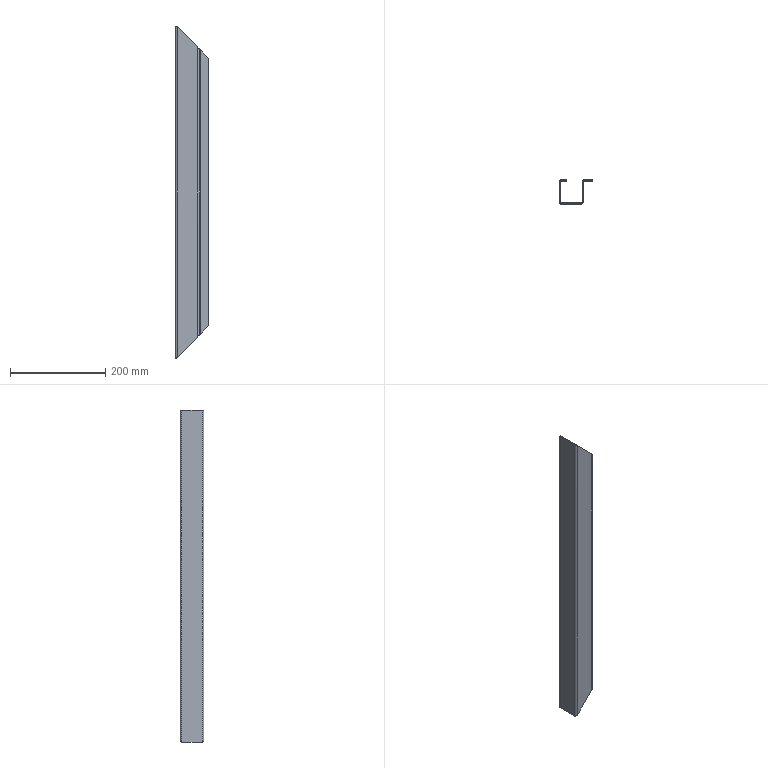Part | STEP file | 750038466 | 1 solid | 38 faces | box 70 x 50 x 696 mm | volume 223669 mm3 | plane 22 | cylinder 8 | spline 8 | commonest cylinder face diameters 4 x4 8 x4
STEP:
#1=CARTESIAN_POINT('',(0.,46.,-348.));
#2=VERTEX_POINT('',#1);
#3=CARTESIAN_POINT('',(0.,4.,-348.));
#4=VERTEX_POINT('',#3);
#5=CARTESIAN_POINT('',(0.,0.,-348.));
#6=DIRECTION('',(0.,-1.,0.));
#7=VECTOR('',#6,1000.);
#8=LINE('',#5,#7);
#9=EDGE_CURVE('',#2,#4,#8,.T.);
#10=ORIENTED_EDGE('',*,*,#9,.T.);
#11=CARTESIAN_POINT('',(0.,4.,348.));
#12=VERTEX_POINT('',#11);
#13=CARTESIAN_POINT('',(0.,4.,350.));
#14=DIRECTION('',(0.,0.,1.));
#15=VECTOR('',#14,1000.);
#16=LINE('',#13,#15);
#17=EDGE_CURVE('',#4,#12,#16,.T.);
#18=ORIENTED_EDGE('',*,*,#17,.T.);
#19=CARTESIAN_POINT('',(0.,46.,348.));
#20=VERTEX_POINT('',#19);
#21=CARTESIAN_POINT('',(0.,0.,348.));
#22=DIRECTION('',(0.,1.,0.));
#23=VECTOR('',#22,1000.);
#24=LINE('',#21,#23);
#25=EDGE_CURVE('',#12,#20,#24,.T.);
#26=ORIENTED_EDGE('',*,*,#25,.T.);
#27=CARTESIAN_POINT('',(0.,46.,350.));
#28=DIRECTION('',(0.,0.,-1.));
#29=VECTOR('',#28,1000.);
#30=LINE('',#27,#29);
#31=EDGE_CURVE('',#20,#2,#30,.T.);
#32=ORIENTED_EDGE('',*,*,#31,.T.);
#33=EDGE_LOOP('',(#10,#18,#26,#32));
#34=FACE_OUTER_BOUND('',#33,.T.);
#35=CARTESIAN_POINT('',(0.,0.,350.));
#36=DIRECTION('',(-1.,0.,0.));
#37=DIRECTION('',(0.,-1.,0.));
#38=AXIS2_PLACEMENT_3D('',#35,#36,#37);
#39=PLANE('',#38);
#40=ADVANCED_FACE('',(#34),#39,.T.);
#41=CARTESIAN_POINT('',(4.,0.,-346.));
#42=VERTEX_POINT('',#41);
#43=CARTESIAN_POINT('',(0.,4.,-348.));
#44=CARTESIAN_POINT('',(0.,2.,-348.));
#45=CARTESIAN_POINT('',(1.333,0.,-347.333));
#46=CARTESIAN_POINT('',(4.,0.,-346.));
#47=(BOUNDED_CURVE()B_SPLINE_CURVE(3,(#43,#44,#45,#46),.UNSPECIFIED.,.F.,.F.)B_SPLINE_CURVE_WITH_KNOTS((4,4),(0.,0.006692),.UNSPECIFIED.)CURVE()GEOMETRIC_REPRESENTATION_ITEM()RATIONAL_B_SPLINE_CURVE((1.,0.6667,0.5,0.5))REPRESENTATION_ITEM(''));
#48=EDGE_CURVE('',#4,#42,#47,.T.);
#49=ORIENTED_EDGE('',*,*,#48,.T.);
#50=CARTESIAN_POINT('',(4.,0.,346.));
#51=VERTEX_POINT('',#50);
#52=CARTESIAN_POINT('',(4.,0.,350.));
#53=DIRECTION('',(0.,0.,1.));
#54=VECTOR('',#53,1000.);
#55=LINE('',#52,#54);
#56=EDGE_CURVE('',#42,#51,#55,.T.);
#57=ORIENTED_EDGE('',*,*,#56,.T.);
#58=CARTESIAN_POINT('',(4.,0.,346.));
#59=CARTESIAN_POINT('',(1.333,0.,347.333));
#60=CARTESIAN_POINT('',(0.,2.,348.));
#61=CARTESIAN_POINT('',(0.,4.,348.));
#62=(BOUNDED_CURVE()B_SPLINE_CURVE(3,(#58,#59,#60,#61),.UNSPECIFIED.,.F.,.F.)B_SPLINE_CURVE_WITH_KNOTS((4,4),(0.,0.006641),.UNSPECIFIED.)CURVE()GEOMETRIC_REPRESENTATION_ITEM()RATIONAL_B_SPLINE_CURVE((0.5,0.5,0.6667,1.))REPRESENTATION_ITEM(''));
#63=EDGE_CURVE('',#51,#12,#62,.T.);
#64=ORIENTED_EDGE('',*,*,#63,.T.);
#65=ORIENTED_EDGE('',*,*,#17,.F.);
#66=EDGE_LOOP('',(#49,#57,#64,#65));
#67=FACE_OUTER_BOUND('',#66,.T.);
#68=CARTESIAN_POINT('',(4.,4.,350.));
#69=DIRECTION('',(0.,0.,-1.));
#70=DIRECTION('',(-1.,0.,0.));
#71=AXIS2_PLACEMENT_3D('',#68,#69,#70);
#72=CYLINDRICAL_SURFACE('',#71,4.);
#73=ADVANCED_FACE('',(#67),#72,.T.);
#74=CARTESIAN_POINT('',(2.,46.,-348.));
#75=VERTEX_POINT('',#74);
#76=CARTESIAN_POINT('',(2.,46.,-348.));
#77=DIRECTION('',(-1.,0.,0.));
#78=VECTOR('',#77,1000.);
#79=LINE('',#76,#78);
#80=EDGE_CURVE('',#75,#2,#79,.T.);
#81=ORIENTED_EDGE('',*,*,#80,.F.);
#82=CARTESIAN_POINT('',(2.,4.,-348.));
#83=VERTEX_POINT('',#82);
#84=CARTESIAN_POINT('',(2.,0.,-348.));
#85=DIRECTION('',(0.,1.,0.));
#86=VECTOR('',#85,1000.);
#87=LINE('',#84,#86);
#88=EDGE_CURVE('',#83,#75,#87,.T.);
#89=ORIENTED_EDGE('',*,*,#88,.F.);
#90=CARTESIAN_POINT('',(2.,4.,-348.));
#91=DIRECTION('',(1.,0.,0.));
#92=VECTOR('',#91,1000.);
#93=LINE('',#90,#92);
#94=EDGE_CURVE('',#4,#83,#93,.T.);
#95=ORIENTED_EDGE('',*,*,#94,.F.);
#96=ORIENTED_EDGE('',*,*,#9,.F.);
#97=EDGE_LOOP('',(#81,#89,#95,#96));
#98=FACE_OUTER_BOUND('',#97,.T.);
#99=CARTESIAN_POINT('',(2.,0.,-348.));
#100=DIRECTION('',(0.,0.,1.));
#101=DIRECTION('',(0.,-1.,0.));
#102=AXIS2_PLACEMENT_3D('',#99,#100,#101);
#103=PLANE('',#102);
#104=ADVANCED_FACE('',(#98),#103,.F.);
#105=CARTESIAN_POINT('',(4.,50.,-346.));
#106=VERTEX_POINT('',#105);
#107=CARTESIAN_POINT('',(4.,50.,-346.));
#108=CARTESIAN_POINT('',(1.333,50.,-347.333));
#109=CARTESIAN_POINT('',(0.,48.,-348.));
#110=CARTESIAN_POINT('',(0.,46.,-348.));
#111=(BOUNDED_CURVE()B_SPLINE_CURVE(3,(#107,#108,#109,#110),.UNSPECIFIED.,.F.,.F.)B_SPLINE_CURVE_WITH_KNOTS((4,4),(0.,0.006641),.UNSPECIFIED.)CURVE()GEOMETRIC_REPRESENTATION_ITEM()RATIONAL_B_SPLINE_CURVE((0.5,0.5,0.6667,1.))REPRESENTATION_ITEM(''));
#112=EDGE_CURVE('',#106,#2,#111,.T.);
#113=ORIENTED_EDGE('',*,*,#112,.T.);
#114=ORIENTED_EDGE('',*,*,#31,.F.);
#115=CARTESIAN_POINT('',(4.,50.,346.));
#116=VERTEX_POINT('',#115);
#117=CARTESIAN_POINT('',(0.,46.,348.));
#118=CARTESIAN_POINT('',(0.,48.,348.));
#119=CARTESIAN_POINT('',(1.333,50.,347.333));
#120=CARTESIAN_POINT('',(4.,50.,346.));
#121=(BOUNDED_CURVE()B_SPLINE_CURVE(3,(#117,#118,#119,#120),.UNSPECIFIED.,.F.,.F.)B_SPLINE_CURVE_WITH_KNOTS((4,4),(0.,0.006627),.UNSPECIFIED.)CURVE()GEOMETRIC_REPRESENTATION_ITEM()RATIONAL_B_SPLINE_CURVE((1.,0.6667,0.5,0.5))REPRESENTATION_ITEM(''));
#122=EDGE_CURVE('',#20,#116,#121,.T.);
#123=ORIENTED_EDGE('',*,*,#122,.T.);
#124=CARTESIAN_POINT('',(4.,50.,350.));
#125=DIRECTION('',(0.,0.,-1.));
#126=VECTOR('',#125,1000.);
#127=LINE('',#124,#126);
#128=EDGE_CURVE('',#116,#106,#127,.T.);
#129=ORIENTED_EDGE('',*,*,#128,.T.);
#130=EDGE_LOOP('',(#113,#114,#123,#129));
#131=FACE_OUTER_BOUND('',#130,.T.);
#132=CARTESIAN_POINT('',(4.,46.,350.));
#133=DIRECTION('',(0.,0.,-1.));
#134=DIRECTION('',(-1.,0.,0.));
#135=AXIS2_PLACEMENT_3D('',#132,#133,#134);
#136=CYLINDRICAL_SURFACE('',#135,4.);
#137=ADVANCED_FACE('',(#131),#136,.T.);
#138=CARTESIAN_POINT('',(2.,46.,348.));
#139=VERTEX_POINT('',#138);
#140=CARTESIAN_POINT('',(2.,4.,348.));
#141=VERTEX_POINT('',#140);
#142=CARTESIAN_POINT('',(2.,0.,348.));
#143=DIRECTION('',(0.,-1.,0.));
#144=VECTOR('',#143,1000.);
#145=LINE('',#142,#144);
#146=EDGE_CURVE('',#139,#141,#145,.T.);
#147=ORIENTED_EDGE('',*,*,#146,.F.);
#148=CARTESIAN_POINT('',(2.,46.,348.));
#149=DIRECTION('',(1.,0.,0.));
#150=VECTOR('',#149,1000.);
#151=LINE('',#148,#150);
#152=EDGE_CURVE('',#20,#139,#151,.T.);
#153=ORIENTED_EDGE('',*,*,#152,.F.);
#154=ORIENTED_EDGE('',*,*,#25,.F.);
#155=CARTESIAN_POINT('',(2.,4.,348.));
#156=DIRECTION('',(-1.,0.,0.));
#157=VECTOR('',#156,1000.);
#158=LINE('',#155,#157);
#159=EDGE_CURVE('',#141,#12,#158,.T.);
#160=ORIENTED_EDGE('',*,*,#159,.F.);
#161=EDGE_LOOP('',(#147,#153,#154,#160));
#162=FACE_OUTER_BOUND('',#161,.T.);
#163=CARTESIAN_POINT('',(2.,0.,348.));
#164=DIRECTION('',(0.,0.,-1.));
#165=DIRECTION('',(0.,1.,0.));
#166=AXIS2_PLACEMENT_3D('',#163,#164,#165);
#167=PLANE('',#166);
#168=ADVANCED_FACE('',(#162),#167,.F.);
#169=CARTESIAN_POINT('',(46.,0.,-304.));
#170=VERTEX_POINT('',#169);
#171=CARTESIAN_POINT('',(4.,0.,-346.));
#172=DIRECTION('',(0.7071,0.,0.7071));
#173=VECTOR('',#172,1000.);
#174=LINE('',#171,#173);
#175=EDGE_CURVE('',#42,#170,#174,.T.);
#176=ORIENTED_EDGE('',*,*,#175,.T.);
#177=CARTESIAN_POINT('',(46.,0.,304.));
#178=VERTEX_POINT('',#177);
#179=CARTESIAN_POINT('',(46.,0.,350.));
#180=DIRECTION('',(0.,0.,1.));
#181=VECTOR('',#180,1000.);
#182=LINE('',#179,#181);
#183=EDGE_CURVE('',#170,#178,#182,.T.);
#184=ORIENTED_EDGE('',*,*,#183,.T.);
#185=CARTESIAN_POINT('',(46.,0.,304.));
#186=DIRECTION('',(-0.7071,0.,0.7071));
#187=VECTOR('',#186,1000.);
#188=LINE('',#185,#187);
#189=EDGE_CURVE('',#178,#51,#188,.T.);
#190=ORIENTED_EDGE('',*,*,#189,.T.);
#191=ORIENTED_EDGE('',*,*,#56,.F.);
#192=EDGE_LOOP('',(#176,#184,#190,#191));
#193=FACE_OUTER_BOUND('',#192,.T.);
#194=CARTESIAN_POINT('',(50.,0.,350.));
#195=DIRECTION('',(0.,-1.,0.));
#196=DIRECTION('',(0.,0.,-1.));
#197=AXIS2_PLACEMENT_3D('',#194,#195,#196);
#198=PLANE('',#197);
#199=ADVANCED_FACE('',(#193),#198,.T.);
#200=CARTESIAN_POINT('',(4.,2.,-346.));
#201=VERTEX_POINT('',#200);
#202=CARTESIAN_POINT('',(4.,1.,-346.));
#203=DIRECTION('',(0.,-1.,0.));
#204=VECTOR('',#203,1000.);
#205=LINE('',#202,#204);
#206=EDGE_CURVE('',#201,#42,#205,.T.);
#207=ORIENTED_EDGE('',*,*,#206,.T.);
#208=ORIENTED_EDGE('',*,*,#48,.F.);
#209=ORIENTED_EDGE('',*,*,#94,.T.);
#210=CARTESIAN_POINT('',(2.,4.,-348.));
#211=CARTESIAN_POINT('',(2.,3.,-348.));
#212=CARTESIAN_POINT('',(2.667,2.,-347.333));
#213=CARTESIAN_POINT('',(4.,2.,-346.));
#214=(BOUNDED_CURVE()B_SPLINE_CURVE(3,(#210,#211,#212,#213),.UNSPECIFIED.,.F.,.F.)B_SPLINE_CURVE_WITH_KNOTS((4,4),(0.,0.003854),.UNSPECIFIED.)CURVE()GEOMETRIC_REPRESENTATION_ITEM()RATIONAL_B_SPLINE_CURVE((1.,0.6667,0.5,0.5))REPRESENTATION_ITEM(''));
#215=EDGE_CURVE('',#83,#201,#214,.T.);
#216=ORIENTED_EDGE('',*,*,#215,.T.);
#217=EDGE_LOOP('',(#207,#208,#209,#216));
#218=FACE_OUTER_BOUND('',#217,.T.);
#219=CARTESIAN_POINT('',(0.,4.,-348.));
#220=CARTESIAN_POINT('',(0.6667,4.,-348.));
#221=CARTESIAN_POINT('',(1.333,4.,-348.));
#222=CARTESIAN_POINT('',(2.,4.,-348.));
#223=CARTESIAN_POINT('',(0.,12.,-348.));
#224=CARTESIAN_POINT('',(0.6667,10.667,-348.));
#225=CARTESIAN_POINT('',(1.333,9.333,-348.));
#226=CARTESIAN_POINT('',(2.,8.,-348.));
#227=CARTESIAN_POINT('',(8.,12.,-344.));
#228=CARTESIAN_POINT('',(7.333,10.667,-344.));
#229=CARTESIAN_POINT('',(6.667,9.333,-344.));
#230=CARTESIAN_POINT('',(6.,8.,-344.));
#231=CARTESIAN_POINT('',(8.,4.,-344.));
#232=CARTESIAN_POINT('',(7.333,4.,-344.));
#233=CARTESIAN_POINT('',(6.667,4.,-344.));
#234=CARTESIAN_POINT('',(6.,4.,-344.));
#235=CARTESIAN_POINT('',(8.,-4.,-344.));
#236=CARTESIAN_POINT('',(7.333,-2.667,-344.));
#237=CARTESIAN_POINT('',(6.667,-1.333,-344.));
#238=CARTESIAN_POINT('',(6.,0.,-344.));
#239=CARTESIAN_POINT('',(0.,-4.,-348.));
#240=CARTESIAN_POINT('',(0.6667,-2.667,-348.));
#241=CARTESIAN_POINT('',(1.333,-1.333,-348.));
#242=CARTESIAN_POINT('',(2.,0.,-348.));
#243=CARTESIAN_POINT('',(0.,4.,-348.));
#244=CARTESIAN_POINT('',(0.6667,4.,-348.));
#245=CARTESIAN_POINT('',(1.333,4.,-348.));
#246=CARTESIAN_POINT('',(2.,4.,-348.));
#247=(BOUNDED_SURFACE()B_SPLINE_SURFACE(3,3,((#219,#220,#221,#222),(#223,#224,#225,#226),(#227,#228,#229,#230),(#231,#232,#233,#234),(#235,#236,#237,#238),(#239,#240,#241,#242),(#243,#244,#245,#246)),.UNSPECIFIED.,.T.,.F.,.F.)B_SPLINE_SURFACE_WITH_KNOTS((4,3,4),(4,4),(0.,0.5,1.),(0.,1.),.UNSPECIFIED.)GEOMETRIC_REPRESENTATION_ITEM()RATIONAL_B_SPLINE_SURFACE(((1.,1.,1.,1.),(0.3333,0.3333,0.3333,0.3333),(0.3333,0.3333,0.3333,0.3333),(1.,1.,1.,1.),(0.3333,0.3333,0.3333,0.3333),(0.3333,0.3333,0.3333,0.3333),(1.,1.,1.,1.)))REPRESENTATION_ITEM('')SURFACE());
#248=ADVANCED_FACE('',(#218),#247,.T.);
#249=ORIENTED_EDGE('',*,*,#159,.T.);
#250=ORIENTED_EDGE('',*,*,#63,.F.);
#251=CARTESIAN_POINT('',(4.,2.,346.));
#252=VERTEX_POINT('',#251);
#253=CARTESIAN_POINT('',(4.,1.,346.));
#254=DIRECTION('',(0.,1.,0.));
#255=VECTOR('',#254,1000.);
#256=LINE('',#253,#255);
#257=EDGE_CURVE('',#51,#252,#256,.T.);
#258=ORIENTED_EDGE('',*,*,#257,.T.);
#259=CARTESIAN_POINT('',(4.,2.,346.));
#260=CARTESIAN_POINT('',(2.667,2.,347.333));
#261=CARTESIAN_POINT('',(2.,3.,348.));
#262=CARTESIAN_POINT('',(2.,4.,348.));
#263=(BOUNDED_CURVE()B_SPLINE_CURVE(3,(#259,#260,#261,#262),.UNSPECIFIED.,.F.,.F.)B_SPLINE_CURVE_WITH_KNOTS((4,4),(0.,0.003785),.UNSPECIFIED.)CURVE()GEOMETRIC_REPRESENTATION_ITEM()RATIONAL_B_SPLINE_CURVE((0.5,0.5,0.6667,1.))REPRESENTATION_ITEM(''));
#264=EDGE_CURVE('',#252,#141,#263,.T.);
#265=ORIENTED_EDGE('',*,*,#264,.T.);
#266=EDGE_LOOP('',(#249,#250,#258,#265));
#267=FACE_OUTER_BOUND('',#266,.T.);
#268=CARTESIAN_POINT('',(8.,4.,344.));
#269=CARTESIAN_POINT('',(7.333,4.,344.));
#270=CARTESIAN_POINT('',(6.667,4.,344.));
#271=CARTESIAN_POINT('',(6.,4.,344.));
#272=CARTESIAN_POINT('',(8.,12.,344.));
#273=CARTESIAN_POINT('',(7.333,10.667,344.));
#274=CARTESIAN_POINT('',(6.667,9.333,344.));
#275=CARTESIAN_POINT('',(6.,8.,344.));
#276=CARTESIAN_POINT('',(0.,12.,348.));
#277=CARTESIAN_POINT('',(0.6667,10.667,348.));
#278=CARTESIAN_POINT('',(1.333,9.333,348.));
#279=CARTESIAN_POINT('',(2.,8.,348.));
#280=CARTESIAN_POINT('',(0.,4.,348.));
#281=CARTESIAN_POINT('',(0.6667,4.,348.));
#282=CARTESIAN_POINT('',(1.333,4.,348.));
#283=CARTESIAN_POINT('',(2.,4.,348.));
#284=CARTESIAN_POINT('',(0.,-4.,348.));
#285=CARTESIAN_POINT('',(0.6667,-2.667,348.));
#286=CARTESIAN_POINT('',(1.333,-1.333,348.));
#287=CARTESIAN_POINT('',(2.,0.,348.));
#288=CARTESIAN_POINT('',(8.,-4.,344.));
#289=CARTESIAN_POINT('',(7.333,-2.667,344.));
#290=CARTESIAN_POINT('',(6.667,-1.333,344.));
#291=CARTESIAN_POINT('',(6.,0.,344.));
#292=CARTESIAN_POINT('',(8.,4.,344.));
#293=CARTESIAN_POINT('',(7.333,4.,344.));
#294=CARTESIAN_POINT('',(6.667,4.,344.));
#295=CARTESIAN_POINT('',(6.,4.,344.));
#296=(BOUNDED_SURFACE()B_SPLINE_SURFACE(3,3,((#268,#269,#270,#271),(#272,#273,#274,#275),(#276,#277,#278,#279),(#280,#281,#282,#283),(#284,#285,#286,#287),(#288,#289,#290,#291),(#292,#293,#294,#295)),.UNSPECIFIED.,.T.,.F.,.F.)B_SPLINE_SURFACE_WITH_KNOTS((4,3,4),(4,4),(0.,0.5,1.),(0.,1.),.UNSPECIFIED.)GEOMETRIC_REPRESENTATION_ITEM()RATIONAL_B_SPLINE_SURFACE(((1.,1.,1.,1.),(0.3333,0.3333,0.3333,0.3333),(0.3333,0.3333,0.3333,0.3333),(1.,1.,1.,1.),(0.3333,0.3333,0.3333,0.3333),(0.3333,0.3333,0.3333,0.3333),(1.,1.,1.,1.)))REPRESENTATION_ITEM('')SURFACE());
#297=ADVANCED_FACE('',(#267),#296,.T.);
#298=ORIENTED_EDGE('',*,*,#80,.T.);
#299=ORIENTED_EDGE('',*,*,#112,.F.);
#300=CARTESIAN_POINT('',(4.,48.,-346.));
#301=VERTEX_POINT('',#300);
#302=CARTESIAN_POINT('',(4.,49.,-346.));
#303=DIRECTION('',(0.,-1.,0.));
#304=VECTOR('',#303,1000.);
#305=LINE('',#302,#304);
#306=EDGE_CURVE('',#106,#301,#305,.T.);
#307=ORIENTED_EDGE('',*,*,#306,.T.);
#308=CARTESIAN_POINT('',(4.,48.,-346.));
#309=CARTESIAN_POINT('',(2.667,48.,-347.333));
#310=CARTESIAN_POINT('',(2.,47.,-348.));
#311=CARTESIAN_POINT('',(2.,46.,-348.));
#312=(BOUNDED_CURVE()B_SPLINE_CURVE(3,(#308,#309,#310,#311),.UNSPECIFIED.,.F.,.T.)B_SPLINE_CURVE_WITH_KNOTS((4,4),(0.,0.003785),.UNSPECIFIED.)CURVE()GEOMETRIC_REPRESENTATION_ITEM()RATIONAL_B_SPLINE_CURVE((0.5,0.5,0.6667,1.))REPRESENTATION_ITEM(''));
#313=EDGE_CURVE('',#301,#75,#312,.T.);
#314=ORIENTED_EDGE('',*,*,#313,.T.);
#315=EDGE_LOOP('',(#298,#299,#307,#314));
#316=FACE_OUTER_BOUND('',#315,.T.);
#317=CARTESIAN_POINT('',(0.,46.,-348.));
#318=CARTESIAN_POINT('',(0.6667,46.,-348.));
#319=CARTESIAN_POINT('',(1.333,46.,-348.));
#320=CARTESIAN_POINT('',(2.,46.,-348.));
#321=CARTESIAN_POINT('',(0.,54.,-348.));
#322=CARTESIAN_POINT('',(0.6667,52.667,-348.));
#323=CARTESIAN_POINT('',(1.333,51.333,-348.));
#324=CARTESIAN_POINT('',(2.,50.,-348.));
#325=CARTESIAN_POINT('',(8.,54.,-344.));
#326=CARTESIAN_POINT('',(7.333,52.667,-344.));
#327=CARTESIAN_POINT('',(6.667,51.333,-344.));
#328=CARTESIAN_POINT('',(6.,50.,-344.));
#329=CARTESIAN_POINT('',(8.,46.,-344.));
#330=CARTESIAN_POINT('',(7.333,46.,-344.));
#331=CARTESIAN_POINT('',(6.667,46.,-344.));
#332=CARTESIAN_POINT('',(6.,46.,-344.));
#333=CARTESIAN_POINT('',(8.,38.,-344.));
#334=CARTESIAN_POINT('',(7.333,39.333,-344.));
#335=CARTESIAN_POINT('',(6.667,40.667,-344.));
#336=CARTESIAN_POINT('',(6.,42.,-344.));
#337=CARTESIAN_POINT('',(0.,38.,-348.));
#338=CARTESIAN_POINT('',(0.6667,39.333,-348.));
#339=CARTESIAN_POINT('',(1.333,40.667,-348.));
#340=CARTESIAN_POINT('',(2.,42.,-348.));
#341=CARTESIAN_POINT('',(0.,46.,-348.));
#342=CARTESIAN_POINT('',(0.6667,46.,-348.));
#343=CARTESIAN_POINT('',(1.333,46.,-348.));
#344=CARTESIAN_POINT('',(2.,46.,-348.));
#345=(BOUNDED_SURFACE()B_SPLINE_SURFACE(3,3,((#317,#318,#319,#320),(#321,#322,#323,#324),(#325,#326,#327,#328),(#329,#330,#331,#332),(#333,#334,#335,#336),(#337,#338,#339,#340),(#341,#342,#343,#344)),.UNSPECIFIED.,.T.,.F.,.F.)B_SPLINE_SURFACE_WITH_KNOTS((4,3,4),(4,4),(0.,0.5,1.),(0.,1.),.UNSPECIFIED.)GEOMETRIC_REPRESENTATION_ITEM()RATIONAL_B_SPLINE_SURFACE(((1.,1.,1.,1.),(0.3333,0.3333,0.3333,0.3333),(0.3333,0.3333,0.3333,0.3333),(1.,1.,1.,1.),(0.3333,0.3333,0.3333,0.3333),(0.3333,0.3333,0.3333,0.3333),(1.,1.,1.,1.)))REPRESENTATION_ITEM('')SURFACE());
#346=ADVANCED_FACE('',(#316),#345,.T.);
#347=ORIENTED_EDGE('',*,*,#146,.T.);
#348=CARTESIAN_POINT('',(2.,4.,350.));
#349=DIRECTION('',(0.,0.,1.));
#350=VECTOR('',#349,1000.);
#351=LINE('',#348,#350);
#352=EDGE_CURVE('',#83,#141,#351,.T.);
#353=ORIENTED_EDGE('',*,*,#352,.F.);
#354=ORIENTED_EDGE('',*,*,#88,.T.);
#355=CARTESIAN_POINT('',(2.,46.,350.));
#356=DIRECTION('',(0.,0.,-1.));
#357=VECTOR('',#356,1000.);
#358=LINE('',#355,#357);
#359=EDGE_CURVE('',#139,#75,#358,.T.);
#360=ORIENTED_EDGE('',*,*,#359,.F.);
#361=EDGE_LOOP('',(#347,#353,#354,#360));
#362=FACE_OUTER_BOUND('',#361,.T.);
#363=CARTESIAN_POINT('',(2.,0.,350.));
#364=DIRECTION('',(-1.,0.,0.));
#365=DIRECTION('',(0.,-1.,0.));
#366=AXIS2_PLACEMENT_3D('',#363,#364,#365);
#367=PLANE('',#366);
#368=ADVANCED_FACE('',(#362),#367,.F.);
#369=CARTESIAN_POINT('',(15.,50.,-335.));
#370=VERTEX_POINT('',#369);
#371=CARTESIAN_POINT('',(15.,50.,-335.));
#372=DIRECTION('',(-0.7071,0.,-0.7071));
#373=VECTOR('',#372,1000.);
#374=LINE('',#371,#373);
#375=EDGE_CURVE('',#370,#106,#374,.T.);
#376=ORIENTED_EDGE('',*,*,#375,.T.);
#377=ORIENTED_EDGE('',*,*,#128,.F.);
#378=CARTESIAN_POINT('',(15.,50.,335.));
#379=VERTEX_POINT('',#378);
#380=CARTESIAN_POINT('',(4.,50.,346.));
#381=DIRECTION('',(0.7071,0.,-0.7071));
#382=VECTOR('',#381,1000.);
#383=LINE('',#380,#382);
#384=EDGE_CURVE('',#116,#379,#383,.T.);
#385=ORIENTED_EDGE('',*,*,#384,.T.);
#386=CARTESIAN_POINT('',(15.,50.,350.));
#387=DIRECTION('',(0.,0.,-1.));
#388=VECTOR('',#387,1000.);
#389=LINE('',#386,#388);
#390=EDGE_CURVE('',#379,#370,#389,.T.);
#391=ORIENTED_EDGE('',*,*,#390,.T.);
#392=EDGE_LOOP('',(#376,#377,#385,#391));
#393=FACE_OUTER_BOUND('',#392,.T.);
#394=CARTESIAN_POINT('',(0.,50.,350.));
#395=DIRECTION('',(0.,1.,0.));
#396=DIRECTION('',(0.,0.,1.));
#397=AXIS2_PLACEMENT_3D('',#394,#395,#396);
#398=PLANE('',#397);
#399=ADVANCED_FACE('',(#393),#398,.T.);
#400=CARTESIAN_POINT('',(4.,48.,346.));
#401=VERTEX_POINT('',#400);
#402=CARTESIAN_POINT('',(4.,49.,346.));
#403=DIRECTION('',(0.,1.,0.));
#404=VECTOR('',#403,1000.);
#405=LINE('',#402,#404);
#406=EDGE_CURVE('',#401,#116,#405,.T.);
#407=ORIENTED_EDGE('',*,*,#406,.T.);
#408=ORIENTED_EDGE('',*,*,#122,.F.);
#409=ORIENTED_EDGE('',*,*,#152,.T.);
#410=CARTESIAN_POINT('',(2.,46.,348.));
#411=CARTESIAN_POINT('',(2.,47.,348.));
#412=CARTESIAN_POINT('',(2.667,48.,347.333));
#413=CARTESIAN_POINT('',(4.,48.,346.));
#414=(BOUNDED_CURVE()B_SPLINE_CURVE(3,(#410,#411,#412,#413),.UNSPECIFIED.,.F.,.F.)B_SPLINE_CURVE_WITH_KNOTS((4,4),(0.,0.003806),.UNSPECIFIED.)CURVE()GEOMETRIC_REPRESENTATION_ITEM()RATIONAL_B_SPLINE_CURVE((1.,0.6667,0.5,0.5))REPRESENTATION_ITEM(''));
#415=EDGE_CURVE('',#139,#401,#414,.T.);
#416=ORIENTED_EDGE('',*,*,#415,.T.);
#417=EDGE_LOOP('',(#407,#408,#409,#416));
#418=FACE_OUTER_BOUND('',#417,.T.);
#419=CARTESIAN_POINT('',(8.,46.,344.));
#420=CARTESIAN_POINT('',(7.333,46.,344.));
#421=CARTESIAN_POINT('',(6.667,46.,344.));
#422=CARTESIAN_POINT('',(6.,46.,344.));
#423=CARTESIAN_POINT('',(8.,54.,344.));
#424=CARTESIAN_POINT('',(7.333,52.667,344.));
#425=CARTESIAN_POINT('',(6.667,51.333,344.));
#426=CARTESIAN_POINT('',(6.,50.,344.));
#427=CARTESIAN_POINT('',(0.,54.,348.));
#428=CARTESIAN_POINT('',(0.6667,52.667,348.));
#429=CARTESIAN_POINT('',(1.333,51.333,348.));
#430=CARTESIAN_POINT('',(2.,50.,348.));
#431=CARTESIAN_POINT('',(0.,46.,348.));
#432=CARTESIAN_POINT('',(0.6667,46.,348.));
#433=CARTESIAN_POINT('',(1.333,46.,348.));
#434=CARTESIAN_POINT('',(2.,46.,348.));
#435=CARTESIAN_POINT('',(0.,38.,348.));
#436=CARTESIAN_POINT('',(0.6667,39.333,348.));
#437=CARTESIAN_POINT('',(1.333,40.667,348.));
#438=CARTESIAN_POINT('',(2.,42.,348.));
#439=CARTESIAN_POINT('',(8.,38.,344.));
#440=CARTESIAN_POINT('',(7.333,39.333,344.));
#441=CARTESIAN_POINT('',(6.667,40.667,344.));
#442=CARTESIAN_POINT('',(6.,42.,344.));
#443=CARTESIAN_POINT('',(8.,46.,344.));
#444=CARTESIAN_POINT('',(7.333,46.,344.));
#445=CARTESIAN_POINT('',(6.667,46.,344.));
#446=CARTESIAN_POINT('',(6.,46.,344.));
#447=(BOUNDED_SURFACE()B_SPLINE_SURFACE(3,3,((#419,#420,#421,#422),(#423,#424,#425,#426),(#427,#428,#429,#430),(#431,#432,#433,#434),(#435,#436,#437,#438),(#439,#440,#441,#442),(#443,#444,#445,#446)),.UNSPECIFIED.,.T.,.F.,.F.)B_SPLINE_SURFACE_WITH_KNOTS((4,3,4),(4,4),(0.,0.5,1.),(0.,1.),.UNSPECIFIED.)GEOMETRIC_REPRESENTATION_ITEM()RATIONAL_B_SPLINE_SURFACE(((1.,1.,1.,1.),(0.3333,0.3333,0.3333,0.3333),(0.3333,0.3333,0.3333,0.3333),(1.,1.,1.,1.),(0.3333,0.3333,0.3333,0.3333),(0.3333,0.3333,0.3333,0.3333),(1.,1.,1.,1.)))REPRESENTATION_ITEM('')SURFACE());
#448=ADVANCED_FACE('',(#418),#447,.T.);
#449=CARTESIAN_POINT('',(50.,4.,-300.));
#450=VERTEX_POINT('',#449);
#451=CARTESIAN_POINT('',(46.,0.,-304.));
#452=CARTESIAN_POINT('',(48.667,0.,-301.333));
#453=CARTESIAN_POINT('',(50.,2.,-300.));
#454=CARTESIAN_POINT('',(50.,4.,-300.));
#455=(BOUNDED_CURVE()B_SPLINE_CURVE(3,(#451,#452,#453,#454),.UNSPECIFIED.,.F.,.F.)B_SPLINE_CURVE_WITH_KNOTS((4,4),(0.,0.007567),.UNSPECIFIED.)CURVE()GEOMETRIC_REPRESENTATION_ITEM()RATIONAL_B_SPLINE_CURVE((0.5,0.5,0.6667,1.))REPRESENTATION_ITEM(''));
#456=EDGE_CURVE('',#170,#450,#455,.T.);
#457=ORIENTED_EDGE('',*,*,#456,.T.);
#458=CARTESIAN_POINT('',(50.,4.,300.));
#459=VERTEX_POINT('',#458);
#460=CARTESIAN_POINT('',(50.,4.,350.));
#461=DIRECTION('',(0.,0.,1.));
#462=VECTOR('',#461,1000.);
#463=LINE('',#460,#462);
#464=EDGE_CURVE('',#450,#459,#463,.T.);
#465=ORIENTED_EDGE('',*,*,#464,.T.);
#466=CARTESIAN_POINT('',(50.,4.,300.));
#467=CARTESIAN_POINT('',(50.,2.,300.));
#468=CARTESIAN_POINT('',(48.667,0.,301.333));
#469=CARTESIAN_POINT('',(46.,0.,304.));
#470=(BOUNDED_CURVE()B_SPLINE_CURVE(3,(#466,#467,#468,#469),.UNSPECIFIED.,.F.,.F.)B_SPLINE_CURVE_WITH_KNOTS((4,4),(0.,0.007712),.UNSPECIFIED.)CURVE()GEOMETRIC_REPRESENTATION_ITEM()RATIONAL_B_SPLINE_CURVE((1.,0.6667,0.5,0.5))REPRESENTATION_ITEM(''));
#471=EDGE_CURVE('',#459,#178,#470,.T.);
#472=ORIENTED_EDGE('',*,*,#471,.T.);
#473=ORIENTED_EDGE('',*,*,#183,.F.);
#474=EDGE_LOOP('',(#457,#465,#472,#473));
#475=FACE_OUTER_BOUND('',#474,.T.);
#476=CARTESIAN_POINT('',(46.,4.,350.));
#477=DIRECTION('',(0.,0.,-1.));
#478=DIRECTION('',(-1.,0.,0.));
#479=AXIS2_PLACEMENT_3D('',#476,#477,#478);
#480=CYLINDRICAL_SURFACE('',#479,4.);
#481=ADVANCED_FACE('',(#475),#480,.T.);
#482=ORIENTED_EDGE('',*,*,#175,.F.);
#483=ORIENTED_EDGE('',*,*,#206,.F.);
#484=CARTESIAN_POINT('',(46.,2.,-304.));
#485=VERTEX_POINT('',#484);
#486=CARTESIAN_POINT('',(375.,2.,25.));
#487=DIRECTION('',(-0.7071,0.,-0.7071));
#488=VECTOR('',#487,1000.);
#489=LINE('',#486,#488);
#490=EDGE_CURVE('',#485,#201,#489,.T.);
#491=ORIENTED_EDGE('',*,*,#490,.F.);
#492=CARTESIAN_POINT('',(46.,0.,-304.));
#493=DIRECTION('',(0.,1.,0.));
#494=VECTOR('',#493,1000.);
#495=LINE('',#492,#494);
#496=EDGE_CURVE('',#170,#485,#495,.T.);
#497=ORIENTED_EDGE('',*,*,#496,.F.);
#498=EDGE_LOOP('',(#482,#483,#491,#497));
#499=FACE_OUTER_BOUND('',#498,.T.);
#500=CARTESIAN_POINT('',(375.,0.,25.));
#501=DIRECTION('',(-0.7071,0.,0.7071));
#502=DIRECTION('',(0.7071,0.,0.7071));
#503=AXIS2_PLACEMENT_3D('',#500,#501,#502);
#504=PLANE('',#503);
#505=ADVANCED_FACE('',(#499),#504,.F.);
#506=ORIENTED_EDGE('',*,*,#189,.F.);
#507=CARTESIAN_POINT('',(46.,2.,304.));
#508=VERTEX_POINT('',#507);
#509=CARTESIAN_POINT('',(46.,0.,304.));
#510=DIRECTION('',(0.,-1.,0.));
#511=VECTOR('',#510,1000.);
#512=LINE('',#509,#511);
#513=EDGE_CURVE('',#508,#178,#512,.T.);
#514=ORIENTED_EDGE('',*,*,#513,.F.);
#515=CARTESIAN_POINT('',(25.,2.,325.));
#516=DIRECTION('',(0.7071,0.,-0.7071));
#517=VECTOR('',#516,1000.);
#518=LINE('',#515,#517);
#519=EDGE_CURVE('',#252,#508,#518,.T.);
#520=ORIENTED_EDGE('',*,*,#519,.F.);
#521=ORIENTED_EDGE('',*,*,#257,.F.);
#522=EDGE_LOOP('',(#506,#514,#520,#521));
#523=FACE_OUTER_BOUND('',#522,.T.);
#524=CARTESIAN_POINT('',(25.,0.,325.));
#525=DIRECTION('',(-0.7071,0.,-0.7071));
#526=DIRECTION('',(-0.7071,0.,0.7071));
#527=AXIS2_PLACEMENT_3D('',#524,#525,#526);
#528=PLANE('',#527);
#529=ADVANCED_FACE('',(#523),#528,.F.);
#530=ORIENTED_EDGE('',*,*,#264,.F.);
#531=CARTESIAN_POINT('',(4.,2.,350.));
#532=DIRECTION('',(0.,0.,1.));
#533=VECTOR('',#532,1000.);
#534=LINE('',#531,#533);
#535=EDGE_CURVE('',#201,#252,#534,.T.);
#536=ORIENTED_EDGE('',*,*,#535,.F.);
#537=ORIENTED_EDGE('',*,*,#215,.F.);
#538=ORIENTED_EDGE('',*,*,#352,.T.);
#539=EDGE_LOOP('',(#530,#536,#537,#538));
#540=FACE_OUTER_BOUND('',#539,.T.);
#541=CARTESIAN_POINT('',(4.,4.,350.));
#542=DIRECTION('',(0.,0.,-1.));
#543=DIRECTION('',(-1.,0.,0.));
#544=AXIS2_PLACEMENT_3D('',#541,#542,#543);
#545=CYLINDRICAL_SURFACE('',#544,2.);
#546=ADVANCED_FACE('',(#540),#545,.F.);
#547=ORIENTED_EDGE('',*,*,#415,.F.);
#548=ORIENTED_EDGE('',*,*,#359,.T.);
#549=ORIENTED_EDGE('',*,*,#313,.F.);
#550=CARTESIAN_POINT('',(4.,48.,350.));
#551=DIRECTION('',(0.,0.,-1.));
#552=VECTOR('',#551,1000.);
#553=LINE('',#550,#552);
#554=EDGE_CURVE('',#401,#301,#553,.T.);
#555=ORIENTED_EDGE('',*,*,#554,.F.);
#556=EDGE_LOOP('',(#547,#548,#549,#555));
#557=FACE_OUTER_BOUND('',#556,.T.);
#558=CARTESIAN_POINT('',(4.,46.,350.));
#559=DIRECTION('',(0.,0.,-1.));
#560=DIRECTION('',(-1.,0.,0.));
#561=AXIS2_PLACEMENT_3D('',#558,#559,#560);
#562=CYLINDRICAL_SURFACE('',#561,2.);
#563=ADVANCED_FACE('',(#557),#562,.F.);
#564=ORIENTED_EDGE('',*,*,#375,.F.);
#565=CARTESIAN_POINT('',(15.,48.,-335.));
#566=VERTEX_POINT('',#565);
#567=CARTESIAN_POINT('',(15.,50.,-335.));
#568=DIRECTION('',(0.,1.,0.));
#569=VECTOR('',#568,1000.);
#570=LINE('',#567,#569);
#571=EDGE_CURVE('',#566,#370,#570,.T.);
#572=ORIENTED_EDGE('',*,*,#571,.F.);
#573=CARTESIAN_POINT('',(350.,48.,0.));
#574=DIRECTION('',(0.7071,0.,0.7071));
#575=VECTOR('',#574,1000.);
#576=LINE('',#573,#575);
#577=EDGE_CURVE('',#301,#566,#576,.T.);
#578=ORIENTED_EDGE('',*,*,#577,.F.);
#579=ORIENTED_EDGE('',*,*,#306,.F.);
#580=EDGE_LOOP('',(#564,#572,#578,#579));
#581=FACE_OUTER_BOUND('',#580,.T.);
#582=CARTESIAN_POINT('',(350.,50.,0.));
#583=DIRECTION('',(-0.7071,0.,0.7071));
#584=DIRECTION('',(0.7071,0.,0.7071));
#585=AXIS2_PLACEMENT_3D('',#582,#583,#584);
#586=PLANE('',#585);
#587=ADVANCED_FACE('',(#581),#586,.F.);
#588=ORIENTED_EDGE('',*,*,#571,.T.);
#589=ORIENTED_EDGE('',*,*,#390,.F.);
#590=CARTESIAN_POINT('',(15.,48.,335.));
#591=VERTEX_POINT('',#590);
#592=CARTESIAN_POINT('',(15.,50.,335.));
#593=DIRECTION('',(0.,-1.,0.));
#594=VECTOR('',#593,1000.);
#595=LINE('',#592,#594);
#596=EDGE_CURVE('',#379,#591,#595,.T.);
#597=ORIENTED_EDGE('',*,*,#596,.T.);
#598=CARTESIAN_POINT('',(15.,48.,350.));
#599=DIRECTION('',(0.,0.,-1.));
#600=VECTOR('',#599,1000.);
#601=LINE('',#598,#600);
#602=EDGE_CURVE('',#591,#566,#601,.T.);
#603=ORIENTED_EDGE('',*,*,#602,.T.);
#604=EDGE_LOOP('',(#588,#589,#597,#603));
#605=FACE_OUTER_BOUND('',#604,.T.);
#606=CARTESIAN_POINT('',(15.,50.,350.));
#607=DIRECTION('',(1.,0.,0.));
#608=DIRECTION('',(0.,0.,-1.));
#609=AXIS2_PLACEMENT_3D('',#606,#607,#608);
#610=PLANE('',#609);
#611=ADVANCED_FACE('',(#605),#610,.T.);
#612=ORIENTED_EDGE('',*,*,#384,.F.);
#613=ORIENTED_EDGE('',*,*,#406,.F.);
#614=CARTESIAN_POINT('',(0.,48.,350.));
#615=DIRECTION('',(-0.7071,0.,0.7071));
#616=VECTOR('',#615,1000.);
#617=LINE('',#614,#616);
#618=EDGE_CURVE('',#591,#401,#617,.T.);
#619=ORIENTED_EDGE('',*,*,#618,.F.);
#620=ORIENTED_EDGE('',*,*,#596,.F.);
#621=EDGE_LOOP('',(#612,#613,#619,#620));
#622=FACE_OUTER_BOUND('',#621,.T.);
#623=CARTESIAN_POINT('',(0.,50.,350.));
#624=DIRECTION('',(-0.7071,0.,-0.7071));
#625=DIRECTION('',(-0.7071,0.,0.7071));
#626=AXIS2_PLACEMENT_3D('',#623,#624,#625);
#627=PLANE('',#626);
#628=ADVANCED_FACE('',(#622),#627,.F.);
#629=CARTESIAN_POINT('',(50.,46.,-300.));
#630=VERTEX_POINT('',#629);
#631=CARTESIAN_POINT('',(50.,48.,-300.));
#632=DIRECTION('',(0.,1.,0.));
#633=VECTOR('',#632,1000.);
#634=LINE('',#631,#633);
#635=EDGE_CURVE('',#450,#630,#634,.T.);
#636=ORIENTED_EDGE('',*,*,#635,.T.);
#637=CARTESIAN_POINT('',(50.,46.,300.));
#638=VERTEX_POINT('',#637);
#639=CARTESIAN_POINT('',(50.,46.,350.));
#640=DIRECTION('',(0.,0.,1.));
#641=VECTOR('',#640,1000.);
#642=LINE('',#639,#641);
#643=EDGE_CURVE('',#630,#638,#642,.T.);
#644=ORIENTED_EDGE('',*,*,#643,.T.);
#645=CARTESIAN_POINT('',(50.,48.,300.));
#646=DIRECTION('',(0.,-1.,0.));
#647=VECTOR('',#646,1000.);
#648=LINE('',#645,#647);
#649=EDGE_CURVE('',#638,#459,#648,.T.);
#650=ORIENTED_EDGE('',*,*,#649,.T.);
#651=ORIENTED_EDGE('',*,*,#464,.F.);
#652=EDGE_LOOP('',(#636,#644,#650,#651));
#653=FACE_OUTER_BOUND('',#652,.T.);
#654=CARTESIAN_POINT('',(50.,48.,350.));
#655=DIRECTION('',(1.,0.,0.));
#656=DIRECTION('',(0.,1.,0.));
#657=AXIS2_PLACEMENT_3D('',#654,#655,#656);
#658=PLANE('',#657);
#659=ADVANCED_FACE('',(#653),#658,.T.);
#660=ORIENTED_EDGE('',*,*,#496,.T.);
#661=CARTESIAN_POINT('',(48.,4.,-300.));
#662=VERTEX_POINT('',#661);
#663=CARTESIAN_POINT('',(46.,2.,-304.));
#664=CARTESIAN_POINT('',(47.333,2.,-301.333));
#665=CARTESIAN_POINT('',(48.,3.,-300.));
#666=CARTESIAN_POINT('',(48.,4.,-300.));
#667=(BOUNDED_CURVE()B_SPLINE_CURVE(3,(#663,#664,#665,#666),.UNSPECIFIED.,.F.,.F.)B_SPLINE_CURVE_WITH_KNOTS((4,4),(0.,0.005228),.UNSPECIFIED.)CURVE()GEOMETRIC_REPRESENTATION_ITEM()RATIONAL_B_SPLINE_CURVE((0.5,0.5,0.6667,1.))REPRESENTATION_ITEM(''));
#668=EDGE_CURVE('',#485,#662,#667,.T.);
#669=ORIENTED_EDGE('',*,*,#668,.T.);
#670=CARTESIAN_POINT('',(49.,4.,-300.));
#671=DIRECTION('',(1.,0.,0.));
#672=VECTOR('',#671,1000.);
#673=LINE('',#670,#672);
#674=EDGE_CURVE('',#662,#450,#673,.T.);
#675=ORIENTED_EDGE('',*,*,#674,.T.);
#676=ORIENTED_EDGE('',*,*,#456,.F.);
#677=EDGE_LOOP('',(#660,#669,#675,#676));
#678=FACE_OUTER_BOUND('',#677,.T.);
#679=CARTESIAN_POINT('',(42.,4.,-308.));
#680=CARTESIAN_POINT('',(42.667,4.,-308.));
#681=CARTESIAN_POINT('',(43.333,4.,-308.));
#682=CARTESIAN_POINT('',(44.,4.,-308.));
#683=CARTESIAN_POINT('',(42.,12.,-308.));
#684=CARTESIAN_POINT('',(42.667,10.667,-308.));
#685=CARTESIAN_POINT('',(43.333,9.333,-308.));
#686=CARTESIAN_POINT('',(44.,8.,-308.));
#687=CARTESIAN_POINT('',(50.,12.,-300.));
#688=CARTESIAN_POINT('',(49.333,10.667,-300.));
#689=CARTESIAN_POINT('',(48.667,9.333,-300.));
#690=CARTESIAN_POINT('',(48.,8.,-300.));
#691=CARTESIAN_POINT('',(50.,4.,-300.));
#692=CARTESIAN_POINT('',(49.333,4.,-300.));
#693=CARTESIAN_POINT('',(48.667,4.,-300.));
#694=CARTESIAN_POINT('',(48.,4.,-300.));
#695=CARTESIAN_POINT('',(50.,-4.,-300.));
#696=CARTESIAN_POINT('',(49.333,-2.667,-300.));
#697=CARTESIAN_POINT('',(48.667,-1.333,-300.));
#698=CARTESIAN_POINT('',(48.,0.,-300.));
#699=CARTESIAN_POINT('',(42.,-4.,-308.));
#700=CARTESIAN_POINT('',(42.667,-2.667,-308.));
#701=CARTESIAN_POINT('',(43.333,-1.333,-308.));
#702=CARTESIAN_POINT('',(44.,0.,-308.));
#703=CARTESIAN_POINT('',(42.,4.,-308.));
#704=CARTESIAN_POINT('',(42.667,4.,-308.));
#705=CARTESIAN_POINT('',(43.333,4.,-308.));
#706=CARTESIAN_POINT('',(44.,4.,-308.));
#707=(BOUNDED_SURFACE()B_SPLINE_SURFACE(3,3,((#679,#680,#681,#682),(#683,#684,#685,#686),(#687,#688,#689,#690),(#691,#692,#693,#694),(#695,#696,#697,#698),(#699,#700,#701,#702),(#703,#704,#705,#706)),.UNSPECIFIED.,.T.,.F.,.T.)B_SPLINE_SURFACE_WITH_KNOTS((4,3,4),(4,4),(0.,0.5,1.),(0.,1.),.UNSPECIFIED.)GEOMETRIC_REPRESENTATION_ITEM()RATIONAL_B_SPLINE_SURFACE(((1.,1.,1.,1.),(0.3333,0.3333,0.3333,0.3333),(0.3333,0.3333,0.3333,0.3333),(1.,1.,1.,1.),(0.3333,0.3333,0.3333,0.3333),(0.3333,0.3333,0.3333,0.3333),(1.,1.,1.,1.)))REPRESENTATION_ITEM('')SURFACE());
#708=ADVANCED_FACE('',(#678),#707,.T.);
#709=CARTESIAN_POINT('',(48.,4.,300.));
#710=VERTEX_POINT('',#709);
#711=CARTESIAN_POINT('',(49.,4.,300.));
#712=DIRECTION('',(-1.,0.,0.));
#713=VECTOR('',#712,1000.);
#714=LINE('',#711,#713);
#715=EDGE_CURVE('',#459,#710,#714,.T.);
#716=ORIENTED_EDGE('',*,*,#715,.T.);
#717=CARTESIAN_POINT('',(48.,4.,300.));
#718=CARTESIAN_POINT('',(48.,3.,300.));
#719=CARTESIAN_POINT('',(47.333,2.,301.333));
#720=CARTESIAN_POINT('',(46.,2.,304.));
#721=(BOUNDED_CURVE()B_SPLINE_CURVE(3,(#717,#718,#719,#720),.UNSPECIFIED.,.F.,.F.)B_SPLINE_CURVE_WITH_KNOTS((4,4),(0.,0.00529),.UNSPECIFIED.)CURVE()GEOMETRIC_REPRESENTATION_ITEM()RATIONAL_B_SPLINE_CURVE((1.,0.6667,0.5,0.5))REPRESENTATION_ITEM(''));
#722=EDGE_CURVE('',#710,#508,#721,.T.);
#723=ORIENTED_EDGE('',*,*,#722,.T.);
#724=ORIENTED_EDGE('',*,*,#513,.T.);
#725=ORIENTED_EDGE('',*,*,#471,.F.);
#726=EDGE_LOOP('',(#716,#723,#724,#725));
#727=FACE_OUTER_BOUND('',#726,.T.);
#728=CARTESIAN_POINT('',(50.,4.,300.));
#729=CARTESIAN_POINT('',(49.333,4.,300.));
#730=CARTESIAN_POINT('',(48.667,4.,300.));
#731=CARTESIAN_POINT('',(48.,4.,300.));
#732=CARTESIAN_POINT('',(50.,12.,300.));
#733=CARTESIAN_POINT('',(49.333,10.667,300.));
#734=CARTESIAN_POINT('',(48.667,9.333,300.));
#735=CARTESIAN_POINT('',(48.,8.,300.));
#736=CARTESIAN_POINT('',(42.,12.,308.));
#737=CARTESIAN_POINT('',(42.667,10.667,308.));
#738=CARTESIAN_POINT('',(43.333,9.333,308.));
#739=CARTESIAN_POINT('',(44.,8.,308.));
#740=CARTESIAN_POINT('',(42.,4.,308.));
#741=CARTESIAN_POINT('',(42.667,4.,308.));
#742=CARTESIAN_POINT('',(43.333,4.,308.));
#743=CARTESIAN_POINT('',(44.,4.,308.));
#744=CARTESIAN_POINT('',(42.,-4.,308.));
#745=CARTESIAN_POINT('',(42.667,-2.667,308.));
#746=CARTESIAN_POINT('',(43.333,-1.333,308.));
#747=CARTESIAN_POINT('',(44.,0.,308.));
#748=CARTESIAN_POINT('',(50.,-4.,300.));
#749=CARTESIAN_POINT('',(49.333,-2.667,300.));
#750=CARTESIAN_POINT('',(48.667,-1.333,300.));
#751=CARTESIAN_POINT('',(48.,0.,300.));
#752=CARTESIAN_POINT('',(50.,4.,300.));
#753=CARTESIAN_POINT('',(49.333,4.,300.));
#754=CARTESIAN_POINT('',(48.667,4.,300.));
#755=CARTESIAN_POINT('',(48.,4.,300.));
#756=(BOUNDED_SURFACE()B_SPLINE_SURFACE(3,3,((#728,#729,#730,#731),(#732,#733,#734,#735),(#736,#737,#738,#739),(#740,#741,#742,#743),(#744,#745,#746,#747),(#748,#749,#750,#751),(#752,#753,#754,#755)),.UNSPECIFIED.,.T.,.F.,.F.)B_SPLINE_SURFACE_WITH_KNOTS((4,3,4),(4,4),(0.,0.5,1.),(0.,1.),.UNSPECIFIED.)GEOMETRIC_REPRESENTATION_ITEM()RATIONAL_B_SPLINE_SURFACE(((1.,1.,1.,1.),(0.3333,0.3333,0.3333,0.3333),(0.3333,0.3333,0.3333,0.3333),(1.,1.,1.,1.),(0.3333,0.3333,0.3333,0.3333),(0.3333,0.3333,0.3333,0.3333),(1.,1.,1.,1.)))REPRESENTATION_ITEM('')SURFACE());
#757=ADVANCED_FACE('',(#727),#756,.T.);
#758=ORIENTED_EDGE('',*,*,#519,.T.);
#759=CARTESIAN_POINT('',(46.,2.,350.));
#760=DIRECTION('',(0.,0.,1.));
#761=VECTOR('',#760,1000.);
#762=LINE('',#759,#761);
#763=EDGE_CURVE('',#485,#508,#762,.T.);
#764=ORIENTED_EDGE('',*,*,#763,.F.);
#765=ORIENTED_EDGE('',*,*,#490,.T.);
#766=ORIENTED_EDGE('',*,*,#535,.T.);
#767=EDGE_LOOP('',(#758,#764,#765,#766));
#768=FACE_OUTER_BOUND('',#767,.T.);
#769=CARTESIAN_POINT('',(50.,2.,350.));
#770=DIRECTION('',(0.,-1.,0.));
#771=DIRECTION('',(0.,0.,-1.));
#772=AXIS2_PLACEMENT_3D('',#769,#770,#771);
#773=PLANE('',#772);
#774=ADVANCED_FACE('',(#768),#773,.F.);
#775=ORIENTED_EDGE('',*,*,#618,.T.);
#776=ORIENTED_EDGE('',*,*,#554,.T.);
#777=ORIENTED_EDGE('',*,*,#577,.T.);
#778=ORIENTED_EDGE('',*,*,#602,.F.);
#779=EDGE_LOOP('',(#775,#776,#777,#778));
#780=FACE_OUTER_BOUND('',#779,.T.);
#781=CARTESIAN_POINT('',(0.,48.,350.));
#782=DIRECTION('',(0.,1.,0.));
#783=DIRECTION('',(0.,0.,1.));
#784=AXIS2_PLACEMENT_3D('',#781,#782,#783);
#785=PLANE('',#784);
#786=ADVANCED_FACE('',(#780),#785,.F.);
#787=ORIENTED_EDGE('',*,*,#643,.F.);
#788=CARTESIAN_POINT('',(52.,48.,-298.));
#789=VERTEX_POINT('',#788);
#790=CARTESIAN_POINT('',(52.,48.,-298.));
#791=CARTESIAN_POINT('',(50.667,48.,-299.333));
#792=CARTESIAN_POINT('',(50.,47.,-300.));
#793=CARTESIAN_POINT('',(50.,46.,-300.));
#794=(BOUNDED_CURVE()B_SPLINE_CURVE(3,(#790,#791,#792,#793),.UNSPECIFIED.,.F.,.T.)B_SPLINE_CURVE_WITH_KNOTS((4,4),(0.,0.003785),.UNSPECIFIED.)CURVE()GEOMETRIC_REPRESENTATION_ITEM()RATIONAL_B_SPLINE_CURVE((0.5,0.5,0.6667,1.))REPRESENTATION_ITEM(''));
#795=EDGE_CURVE('',#789,#630,#794,.T.);
#796=ORIENTED_EDGE('',*,*,#795,.F.);
#797=CARTESIAN_POINT('',(52.,48.,298.));
#798=VERTEX_POINT('',#797);
#799=CARTESIAN_POINT('',(52.,48.,350.));
#800=DIRECTION('',(0.,0.,-1.));
#801=VECTOR('',#800,1000.);
#802=LINE('',#799,#801);
#803=EDGE_CURVE('',#798,#789,#802,.T.);
#804=ORIENTED_EDGE('',*,*,#803,.F.);
#805=CARTESIAN_POINT('',(50.,46.,300.));
#806=CARTESIAN_POINT('',(50.,47.,300.));
#807=CARTESIAN_POINT('',(50.667,48.,299.333));
#808=CARTESIAN_POINT('',(52.,48.,298.));
#809=(BOUNDED_CURVE()B_SPLINE_CURVE(3,(#805,#806,#807,#808),.UNSPECIFIED.,.F.,.F.)B_SPLINE_CURVE_WITH_KNOTS((4,4),(0.,0.003854),.UNSPECIFIED.)CURVE()GEOMETRIC_REPRESENTATION_ITEM()RATIONAL_B_SPLINE_CURVE((1.,0.6667,0.5,0.5))REPRESENTATION_ITEM(''));
#810=EDGE_CURVE('',#638,#798,#809,.T.);
#811=ORIENTED_EDGE('',*,*,#810,.F.);
#812=EDGE_LOOP('',(#787,#796,#804,#811));
#813=FACE_OUTER_BOUND('',#812,.T.);
#814=CARTESIAN_POINT('',(52.,46.,350.));
#815=DIRECTION('',(0.,0.,-1.));
#816=DIRECTION('',(-1.,0.,0.));
#817=AXIS2_PLACEMENT_3D('',#814,#815,#816);
#818=CYLINDRICAL_SURFACE('',#817,2.);
#819=ADVANCED_FACE('',(#813),#818,.F.);
#820=ORIENTED_EDGE('',*,*,#635,.F.);
#821=ORIENTED_EDGE('',*,*,#674,.F.);
#822=CARTESIAN_POINT('',(48.,46.,-300.));
#823=VERTEX_POINT('',#822);
#824=CARTESIAN_POINT('',(48.,48.,-300.));
#825=DIRECTION('',(0.,-1.,0.));
#826=VECTOR('',#825,1000.);
#827=LINE('',#824,#826);
#828=EDGE_CURVE('',#823,#662,#827,.T.);
#829=ORIENTED_EDGE('',*,*,#828,.F.);
#830=CARTESIAN_POINT('',(50.,46.,-300.));
#831=DIRECTION('',(-1.,0.,0.));
#832=VECTOR('',#831,1000.);
#833=LINE('',#830,#832);
#834=EDGE_CURVE('',#630,#823,#833,.T.);
#835=ORIENTED_EDGE('',*,*,#834,.F.);
#836=EDGE_LOOP('',(#820,#821,#829,#835));
#837=FACE_OUTER_BOUND('',#836,.T.);
#838=CARTESIAN_POINT('',(50.,48.,-300.));
#839=DIRECTION('',(0.,0.,1.));
#840=DIRECTION('',(0.,-1.,0.));
#841=AXIS2_PLACEMENT_3D('',#838,#839,#840);
#842=PLANE('',#841);
#843=ADVANCED_FACE('',(#837),#842,.F.);
#844=ORIENTED_EDGE('',*,*,#649,.F.);
#845=CARTESIAN_POINT('',(48.,46.,300.));
#846=VERTEX_POINT('',#845);
#847=CARTESIAN_POINT('',(50.,46.,300.));
#848=DIRECTION('',(1.,0.,0.));
#849=VECTOR('',#848,1000.);
#850=LINE('',#847,#849);
#851=EDGE_CURVE('',#846,#638,#850,.T.);
#852=ORIENTED_EDGE('',*,*,#851,.F.);
#853=CARTESIAN_POINT('',(48.,48.,300.));
#854=DIRECTION('',(0.,1.,0.));
#855=VECTOR('',#854,1000.);
#856=LINE('',#853,#855);
#857=EDGE_CURVE('',#710,#846,#856,.T.);
#858=ORIENTED_EDGE('',*,*,#857,.F.);
#859=ORIENTED_EDGE('',*,*,#715,.F.);
#860=EDGE_LOOP('',(#844,#852,#858,#859));
#861=FACE_OUTER_BOUND('',#860,.T.);
#862=CARTESIAN_POINT('',(50.,48.,300.));
#863=DIRECTION('',(0.,0.,-1.));
#864=DIRECTION('',(0.,1.,0.));
#865=AXIS2_PLACEMENT_3D('',#862,#863,#864);
#866=PLANE('',#865);
#867=ADVANCED_FACE('',(#861),#866,.F.);
#868=ORIENTED_EDGE('',*,*,#722,.F.);
#869=CARTESIAN_POINT('',(48.,4.,350.));
#870=DIRECTION('',(0.,0.,1.));
#871=VECTOR('',#870,1000.);
#872=LINE('',#869,#871);
#873=EDGE_CURVE('',#662,#710,#872,.T.);
#874=ORIENTED_EDGE('',*,*,#873,.F.);
#875=ORIENTED_EDGE('',*,*,#668,.F.);
#876=ORIENTED_EDGE('',*,*,#763,.T.);
#877=EDGE_LOOP('',(#868,#874,#875,#876));
#878=FACE_OUTER_BOUND('',#877,.T.);
#879=CARTESIAN_POINT('',(46.,4.,350.));
#880=DIRECTION('',(0.,0.,-1.));
#881=DIRECTION('',(-1.,0.,0.));
#882=AXIS2_PLACEMENT_3D('',#879,#880,#881);
#883=CYLINDRICAL_SURFACE('',#882,2.);
#884=ADVANCED_FACE('',(#878),#883,.F.);
#885=CARTESIAN_POINT('',(52.,50.,298.));
#886=VERTEX_POINT('',#885);
#887=CARTESIAN_POINT('',(52.,49.,298.));
#888=DIRECTION('',(0.,1.,0.));
#889=VECTOR('',#888,1000.);
#890=LINE('',#887,#889);
#891=EDGE_CURVE('',#798,#886,#890,.T.);
#892=ORIENTED_EDGE('',*,*,#891,.T.);
#893=CARTESIAN_POINT('',(52.,50.,298.));
#894=CARTESIAN_POINT('',(49.333,50.,299.333));
#895=CARTESIAN_POINT('',(48.,48.,300.));
#896=CARTESIAN_POINT('',(48.,46.,300.));
#897=(BOUNDED_CURVE()B_SPLINE_CURVE(3,(#893,#894,#895,#896),.UNSPECIFIED.,.F.,.F.)B_SPLINE_CURVE_WITH_KNOTS((4,4),(0.,0.006622),.UNSPECIFIED.)CURVE()GEOMETRIC_REPRESENTATION_ITEM()RATIONAL_B_SPLINE_CURVE((0.5,0.5,0.6667,1.))REPRESENTATION_ITEM(''));
#898=EDGE_CURVE('',#886,#846,#897,.T.);
#899=ORIENTED_EDGE('',*,*,#898,.T.);
#900=ORIENTED_EDGE('',*,*,#851,.T.);
#901=ORIENTED_EDGE('',*,*,#810,.T.);
#902=EDGE_LOOP('',(#892,#899,#900,#901));
#903=FACE_OUTER_BOUND('',#902,.T.);
#904=CARTESIAN_POINT('',(54.,46.,296.));
#905=CARTESIAN_POINT('',(54.667,46.,296.));
#906=CARTESIAN_POINT('',(55.333,46.,296.));
#907=CARTESIAN_POINT('',(56.,46.,296.));
#908=CARTESIAN_POINT('',(54.,42.,296.));
#909=CARTESIAN_POINT('',(54.667,40.667,296.));
#910=CARTESIAN_POINT('',(55.333,39.333,296.));
#911=CARTESIAN_POINT('',(56.,38.,296.));
#912=CARTESIAN_POINT('',(50.,42.,300.));
#913=CARTESIAN_POINT('',(49.333,40.667,300.));
#914=CARTESIAN_POINT('',(48.667,39.333,300.));
#915=CARTESIAN_POINT('',(48.,38.,300.));
#916=CARTESIAN_POINT('',(50.,46.,300.));
#917=CARTESIAN_POINT('',(49.333,46.,300.));
#918=CARTESIAN_POINT('',(48.667,46.,300.));
#919=CARTESIAN_POINT('',(48.,46.,300.));
#920=CARTESIAN_POINT('',(50.,50.,300.));
#921=CARTESIAN_POINT('',(49.333,51.333,300.));
#922=CARTESIAN_POINT('',(48.667,52.667,300.));
#923=CARTESIAN_POINT('',(48.,54.,300.));
#924=CARTESIAN_POINT('',(54.,50.,296.));
#925=CARTESIAN_POINT('',(54.667,51.333,296.));
#926=CARTESIAN_POINT('',(55.333,52.667,296.));
#927=CARTESIAN_POINT('',(56.,54.,296.));
#928=CARTESIAN_POINT('',(54.,46.,296.));
#929=CARTESIAN_POINT('',(54.667,46.,296.));
#930=CARTESIAN_POINT('',(55.333,46.,296.));
#931=CARTESIAN_POINT('',(56.,46.,296.));
#932=(BOUNDED_SURFACE()B_SPLINE_SURFACE(3,3,((#904,#905,#906,#907),(#908,#909,#910,#911),(#912,#913,#914,#915),(#916,#917,#918,#919),(#920,#921,#922,#923),(#924,#925,#926,#927),(#928,#929,#930,#931)),.UNSPECIFIED.,.T.,.F.,.F.)B_SPLINE_SURFACE_WITH_KNOTS((4,3,4),(4,4),(0.,0.5,1.),(0.,1.),.UNSPECIFIED.)GEOMETRIC_REPRESENTATION_ITEM()RATIONAL_B_SPLINE_SURFACE(((1.,1.,1.,1.),(0.3333,0.3333,0.3333,0.3333),(0.3333,0.3333,0.3333,0.3333),(1.,1.,1.,1.),(0.3333,0.3333,0.3333,0.3333),(0.3333,0.3333,0.3333,0.3333),(1.,1.,1.,1.)))REPRESENTATION_ITEM('')SURFACE());
#933=ADVANCED_FACE('',(#903),#932,.T.);
#934=ORIENTED_EDGE('',*,*,#834,.T.);
#935=CARTESIAN_POINT('',(52.,50.,-298.));
#936=VERTEX_POINT('',#935);
#937=CARTESIAN_POINT('',(48.,46.,-300.));
#938=CARTESIAN_POINT('',(48.,48.,-300.));
#939=CARTESIAN_POINT('',(49.333,50.,-299.333));
#940=CARTESIAN_POINT('',(52.,50.,-298.));
#941=(BOUNDED_CURVE()B_SPLINE_CURVE(3,(#937,#938,#939,#940),.UNSPECIFIED.,.F.,.F.)B_SPLINE_CURVE_WITH_KNOTS((4,4),(0.,0.006696),.UNSPECIFIED.)CURVE()GEOMETRIC_REPRESENTATION_ITEM()RATIONAL_B_SPLINE_CURVE((1.,0.6667,0.5,0.5))REPRESENTATION_ITEM(''));
#942=EDGE_CURVE('',#823,#936,#941,.T.);
#943=ORIENTED_EDGE('',*,*,#942,.T.);
#944=CARTESIAN_POINT('',(52.,49.,-298.));
#945=DIRECTION('',(0.,-1.,0.));
#946=VECTOR('',#945,1000.);
#947=LINE('',#944,#946);
#948=EDGE_CURVE('',#936,#789,#947,.T.);
#949=ORIENTED_EDGE('',*,*,#948,.T.);
#950=ORIENTED_EDGE('',*,*,#795,.T.);
#951=EDGE_LOOP('',(#934,#943,#949,#950));
#952=FACE_OUTER_BOUND('',#951,.T.);
#953=CARTESIAN_POINT('',(50.,46.,-300.));
#954=CARTESIAN_POINT('',(49.333,46.,-300.));
#955=CARTESIAN_POINT('',(48.667,46.,-300.));
#956=CARTESIAN_POINT('',(48.,46.,-300.));
#957=CARTESIAN_POINT('',(50.,42.,-300.));
#958=CARTESIAN_POINT('',(49.333,40.667,-300.));
#959=CARTESIAN_POINT('',(48.667,39.333,-300.));
#960=CARTESIAN_POINT('',(48.,38.,-300.));
#961=CARTESIAN_POINT('',(54.,42.,-296.));
#962=CARTESIAN_POINT('',(54.667,40.667,-296.));
#963=CARTESIAN_POINT('',(55.333,39.333,-296.));
#964=CARTESIAN_POINT('',(56.,38.,-296.));
#965=CARTESIAN_POINT('',(54.,46.,-296.));
#966=CARTESIAN_POINT('',(54.667,46.,-296.));
#967=CARTESIAN_POINT('',(55.333,46.,-296.));
#968=CARTESIAN_POINT('',(56.,46.,-296.));
#969=CARTESIAN_POINT('',(54.,50.,-296.));
#970=CARTESIAN_POINT('',(54.667,51.333,-296.));
#971=CARTESIAN_POINT('',(55.333,52.667,-296.));
#972=CARTESIAN_POINT('',(56.,54.,-296.));
#973=CARTESIAN_POINT('',(50.,50.,-300.));
#974=CARTESIAN_POINT('',(49.333,51.333,-300.));
#975=CARTESIAN_POINT('',(48.667,52.667,-300.));
#976=CARTESIAN_POINT('',(48.,54.,-300.));
#977=CARTESIAN_POINT('',(50.,46.,-300.));
#978=CARTESIAN_POINT('',(49.333,46.,-300.));
#979=CARTESIAN_POINT('',(48.667,46.,-300.));
#980=CARTESIAN_POINT('',(48.,46.,-300.));
#981=(BOUNDED_SURFACE()B_SPLINE_SURFACE(3,3,((#953,#954,#955,#956),(#957,#958,#959,#960),(#961,#962,#963,#964),(#965,#966,#967,#968),(#969,#970,#971,#972),(#973,#974,#975,#976),(#977,#978,#979,#980)),.UNSPECIFIED.,.T.,.F.,.F.)B_SPLINE_SURFACE_WITH_KNOTS((4,3,4),(4,4),(0.,0.5,1.),(0.,1.),.UNSPECIFIED.)GEOMETRIC_REPRESENTATION_ITEM()RATIONAL_B_SPLINE_SURFACE(((1.,1.,1.,1.),(0.3333,0.3333,0.3333,0.3333),(0.3333,0.3333,0.3333,0.3333),(1.,1.,1.,1.),(0.3333,0.3333,0.3333,0.3333),(0.3333,0.3333,0.3333,0.3333),(1.,1.,1.,1.)))REPRESENTATION_ITEM('')SURFACE());
#982=ADVANCED_FACE('',(#952),#981,.T.);
#983=CARTESIAN_POINT('',(70.,48.,-280.));
#984=VERTEX_POINT('',#983);
#985=CARTESIAN_POINT('',(52.,48.,-298.));
#986=DIRECTION('',(0.7071,0.,0.7071));
#987=VECTOR('',#986,1000.);
#988=LINE('',#985,#987);
#989=EDGE_CURVE('',#789,#984,#988,.T.);
#990=ORIENTED_EDGE('',*,*,#989,.T.);
#991=CARTESIAN_POINT('',(70.,48.,280.));
#992=VERTEX_POINT('',#991);
#993=CARTESIAN_POINT('',(70.,48.,350.));
#994=DIRECTION('',(0.,0.,1.));
#995=VECTOR('',#994,1000.);
#996=LINE('',#993,#995);
#997=EDGE_CURVE('',#984,#992,#996,.T.);
#998=ORIENTED_EDGE('',*,*,#997,.T.);
#999=CARTESIAN_POINT('',(70.,48.,280.));
#1000=DIRECTION('',(-0.7071,0.,0.7071));
#1001=VECTOR('',#1000,1000.);
#1002=LINE('',#999,#1001);
#1003=EDGE_CURVE('',#992,#798,#1002,.T.);
#1004=ORIENTED_EDGE('',*,*,#1003,.T.);
#1005=ORIENTED_EDGE('',*,*,#803,.T.);
#1006=EDGE_LOOP('',(#990,#998,#1004,#1005));
#1007=FACE_OUTER_BOUND('',#1006,.T.);
#1008=CARTESIAN_POINT('',(70.,48.,350.));
#1009=DIRECTION('',(0.,-1.,0.));
#1010=DIRECTION('',(0.,0.,-1.));
#1011=AXIS2_PLACEMENT_3D('',#1008,#1009,#1010);
#1012=PLANE('',#1011);
#1013=ADVANCED_FACE('',(#1007),#1012,.T.);
#1014=ORIENTED_EDGE('',*,*,#857,.T.);
#1015=CARTESIAN_POINT('',(48.,46.,350.));
#1016=DIRECTION('',(0.,0.,1.));
#1017=VECTOR('',#1016,1000.);
#1018=LINE('',#1015,#1017);
#1019=EDGE_CURVE('',#823,#846,#1018,.T.);
#1020=ORIENTED_EDGE('',*,*,#1019,.F.);
#1021=ORIENTED_EDGE('',*,*,#828,.T.);
#1022=ORIENTED_EDGE('',*,*,#873,.T.);
#1023=EDGE_LOOP('',(#1014,#1020,#1021,#1022));
#1024=FACE_OUTER_BOUND('',#1023,.T.);
#1025=CARTESIAN_POINT('',(48.,48.,350.));
#1026=DIRECTION('',(1.,0.,0.));
#1027=DIRECTION('',(0.,1.,0.));
#1028=AXIS2_PLACEMENT_3D('',#1025,#1026,#1027);
#1029=PLANE('',#1028);
#1030=ADVANCED_FACE('',(#1024),#1029,.F.);
#1031=CARTESIAN_POINT('',(52.,50.,350.));
#1032=DIRECTION('',(0.,0.,-1.));
#1033=VECTOR('',#1032,1000.);
#1034=LINE('',#1031,#1033);
#1035=EDGE_CURVE('',#886,#936,#1034,.T.);
#1036=ORIENTED_EDGE('',*,*,#1035,.T.);
#1037=ORIENTED_EDGE('',*,*,#942,.F.);
#1038=ORIENTED_EDGE('',*,*,#1019,.T.);
#1039=ORIENTED_EDGE('',*,*,#898,.F.);
#1040=EDGE_LOOP('',(#1036,#1037,#1038,#1039));
#1041=FACE_OUTER_BOUND('',#1040,.T.);
#1042=CARTESIAN_POINT('',(52.,46.,350.));
#1043=DIRECTION('',(0.,0.,-1.));
#1044=DIRECTION('',(-1.,0.,0.));
#1045=AXIS2_PLACEMENT_3D('',#1042,#1043,#1044);
#1046=CYLINDRICAL_SURFACE('',#1045,4.);
#1047=ADVANCED_FACE('',(#1041),#1046,.T.);
#1048=ORIENTED_EDGE('',*,*,#891,.F.);
#1049=ORIENTED_EDGE('',*,*,#1003,.F.);
#1050=CARTESIAN_POINT('',(70.,50.,280.));
#1051=VERTEX_POINT('',#1050);
#1052=CARTESIAN_POINT('',(70.,48.,280.));
#1053=DIRECTION('',(0.,-1.,0.));
#1054=VECTOR('',#1053,1000.);
#1055=LINE('',#1052,#1054);
#1056=EDGE_CURVE('',#1051,#992,#1055,.T.);
#1057=ORIENTED_EDGE('',*,*,#1056,.F.);
#1058=CARTESIAN_POINT('',(35.,50.,315.));
#1059=DIRECTION('',(0.7071,0.,-0.7071));
#1060=VECTOR('',#1059,1000.);
#1061=LINE('',#1058,#1060);
#1062=EDGE_CURVE('',#886,#1051,#1061,.T.);
#1063=ORIENTED_EDGE('',*,*,#1062,.F.);
#1064=EDGE_LOOP('',(#1048,#1049,#1057,#1063));
#1065=FACE_OUTER_BOUND('',#1064,.T.);
#1066=CARTESIAN_POINT('',(35.,48.,315.));
#1067=DIRECTION('',(-0.7071,0.,-0.7071));
#1068=DIRECTION('',(-0.7071,0.,0.7071));
#1069=AXIS2_PLACEMENT_3D('',#1066,#1067,#1068);
#1070=PLANE('',#1069);
#1071=ADVANCED_FACE('',(#1065),#1070,.F.);
#1072=ORIENTED_EDGE('',*,*,#989,.F.);
#1073=ORIENTED_EDGE('',*,*,#948,.F.);
#1074=CARTESIAN_POINT('',(70.,50.,-280.));
#1075=VERTEX_POINT('',#1074);
#1076=CARTESIAN_POINT('',(385.,50.,35.));
#1077=DIRECTION('',(-0.7071,0.,-0.7071));
#1078=VECTOR('',#1077,1000.);
#1079=LINE('',#1076,#1078);
#1080=EDGE_CURVE('',#1075,#936,#1079,.T.);
#1081=ORIENTED_EDGE('',*,*,#1080,.F.);
#1082=CARTESIAN_POINT('',(70.,48.,-280.));
#1083=DIRECTION('',(0.,1.,0.));
#1084=VECTOR('',#1083,1000.);
#1085=LINE('',#1082,#1084);
#1086=EDGE_CURVE('',#984,#1075,#1085,.T.);
#1087=ORIENTED_EDGE('',*,*,#1086,.F.);
#1088=EDGE_LOOP('',(#1072,#1073,#1081,#1087));
#1089=FACE_OUTER_BOUND('',#1088,.T.);
#1090=CARTESIAN_POINT('',(385.,48.,35.));
#1091=DIRECTION('',(-0.7071,0.,0.7071));
#1092=DIRECTION('',(0.7071,0.,0.7071));
#1093=AXIS2_PLACEMENT_3D('',#1090,#1091,#1092);
#1094=PLANE('',#1093);
#1095=ADVANCED_FACE('',(#1089),#1094,.F.);
#1096=ORIENTED_EDGE('',*,*,#1056,.T.);
#1097=ORIENTED_EDGE('',*,*,#997,.F.);
#1098=ORIENTED_EDGE('',*,*,#1086,.T.);
#1099=CARTESIAN_POINT('',(70.,50.,350.));
#1100=DIRECTION('',(0.,0.,-1.));
#1101=VECTOR('',#1100,1000.);
#1102=LINE('',#1099,#1101);
#1103=EDGE_CURVE('',#1051,#1075,#1102,.T.);
#1104=ORIENTED_EDGE('',*,*,#1103,.F.);
#1105=EDGE_LOOP('',(#1096,#1097,#1098,#1104));
#1106=FACE_OUTER_BOUND('',#1105,.T.);
#1107=CARTESIAN_POINT('',(70.,48.,350.));
#1108=DIRECTION('',(-1.,0.,0.));
#1109=DIRECTION('',(0.,0.,1.));
#1110=AXIS2_PLACEMENT_3D('',#1107,#1108,#1109);
#1111=PLANE('',#1110);
#1112=ADVANCED_FACE('',(#1106),#1111,.F.);
#1113=ORIENTED_EDGE('',*,*,#1062,.T.);
#1114=ORIENTED_EDGE('',*,*,#1103,.T.);
#1115=ORIENTED_EDGE('',*,*,#1080,.T.);
#1116=ORIENTED_EDGE('',*,*,#1035,.F.);
#1117=EDGE_LOOP('',(#1113,#1114,#1115,#1116));
#1118=FACE_OUTER_BOUND('',#1117,.T.);
#1119=CARTESIAN_POINT('',(70.,50.,350.));
#1120=DIRECTION('',(0.,-1.,0.));
#1121=DIRECTION('',(0.,0.,-1.));
#1122=AXIS2_PLACEMENT_3D('',#1119,#1120,#1121);
#1123=PLANE('',#1122);
#1124=ADVANCED_FACE('',(#1118),#1123,.F.);
#1125=CLOSED_SHELL('',(#40,#73,#104,#137,#168,#199,#248,#297,#346,#368,#399,#448,#481,#505,#529,#546,#563,#587,#611,#628,#659,#708,#757,#774,#786,#819,#843,#867,#884,#933,#982,#1013,#1030,#1047,#1071,#1095,#1112,#1124));
#1126=MANIFOLD_SOLID_BREP('',#1125);
#1127=CARTESIAN_POINT('',(0.,0.,0.));
#1128=DIRECTION('',(0.,0.,1.));
#1129=DIRECTION('',(1.,0.,0.));
#1130=AXIS2_PLACEMENT_3D('',#1127,#1128,#1129);
#1131=(LENGTH_UNIT()NAMED_UNIT(*)SI_UNIT(.MILLI.,.METRE.));
#1132=UNCERTAINTY_MEASURE_WITH_UNIT(LENGTH_MEASURE(0.00001),#1131,'','');
#1133=(NAMED_UNIT(*)PLANE_ANGLE_UNIT()SI_UNIT($,.RADIAN.));
#1134=(NAMED_UNIT(*)SI_UNIT($,.STERADIAN.)SOLID_ANGLE_UNIT());
#1135=(GEOMETRIC_REPRESENTATION_CONTEXT(3)GLOBAL_UNCERTAINTY_ASSIGNED_CONTEXT((#1132))GLOBAL_UNIT_ASSIGNED_CONTEXT((#1131,#1133,#1134))REPRESENTATION_CONTEXT('',''));
#1136=ADVANCED_BREP_SHAPE_REPRESENTATION('',(#1126,#1130),#1135);